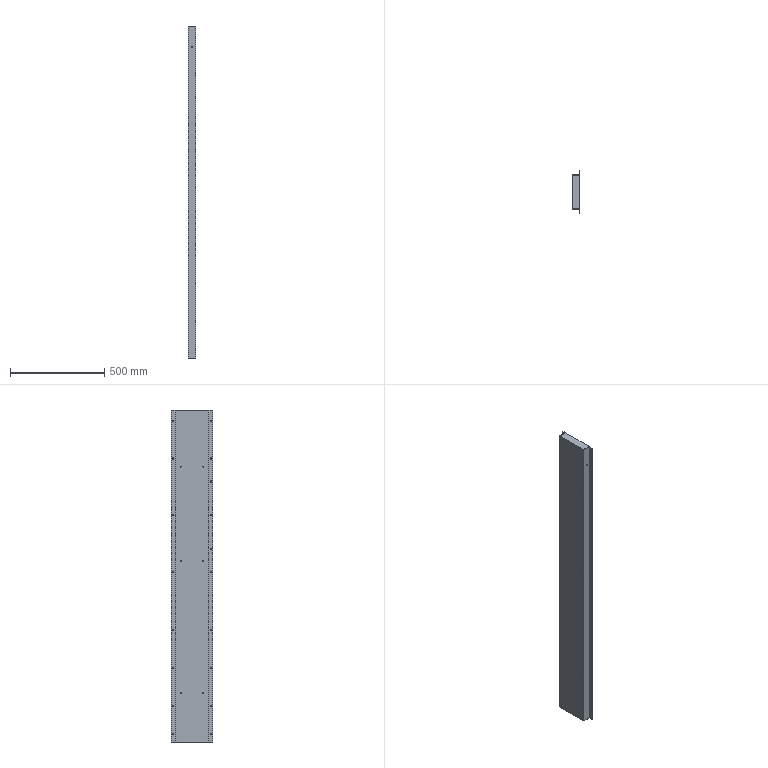Part | SolidWorks | features BaseBody 1 | 1 solid | 86 faces | box 42 x 220 x 1760 mm | volume 1067882 mm3 | cylinder 52 | plane 34 | commonest cylinder face diameters 6.5 x36 5.5 x12 9 x4